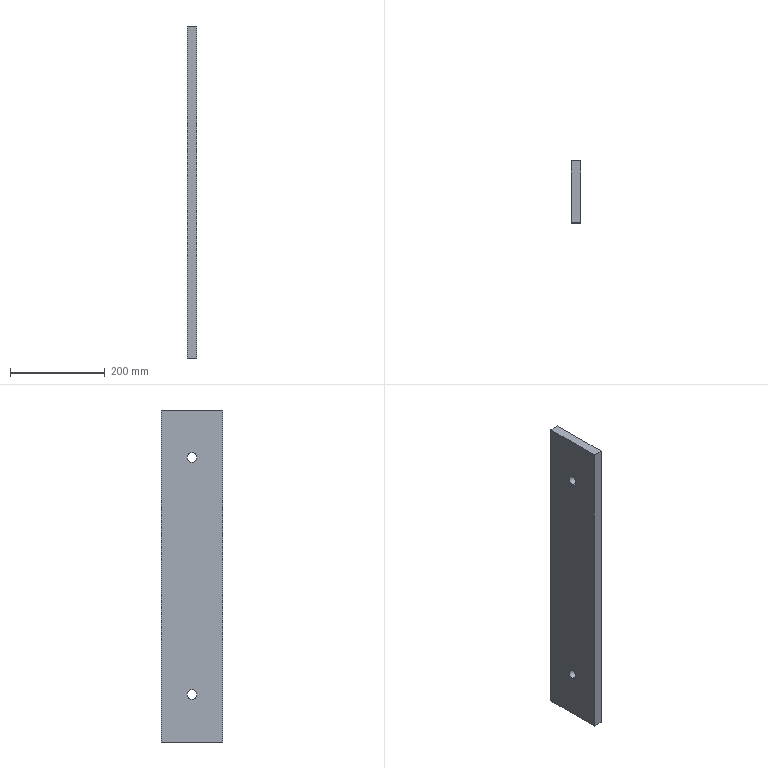Part | SolidWorks | features Extrusion 1 | 1 solid | 10 faces | box 20 x 130 x 700 mm | volume 1807434 mm3 | plane 6 | cylinder 4 | commonest cylinder face diameters 20 x4
STEP:
#1=CARTESIAN_POINT('',(20.,0.,-240.));
#2=VERTEX_POINT('',#1);
#3=CARTESIAN_POINT('',(20.,0.,-260.));
#4=VERTEX_POINT('',#3);
#5=CARTESIAN_POINT('',(20.,0.,-250.));
#6=DIRECTION('',(1.,0.,0.));
#7=DIRECTION('',(0.,0.,-1.));
#8=AXIS2_PLACEMENT_3D('',#5,#6,#7);
#9=CIRCLE('',#8,10.);
#10=EDGE_CURVE('',#2,#4,#9,.T.);
#11=ORIENTED_EDGE('',*,*,#10,.T.);
#12=CARTESIAN_POINT('',(0.,0.,-260.));
#13=VERTEX_POINT('',#12);
#14=CARTESIAN_POINT('',(20.,0.,-260.));
#15=DIRECTION('',(-1.,0.,0.));
#16=VECTOR('',#15,1000.);
#17=LINE('',#14,#16);
#18=EDGE_CURVE('',#4,#13,#17,.T.);
#19=ORIENTED_EDGE('',*,*,#18,.T.);
#20=CARTESIAN_POINT('',(0.,0.,-240.));
#21=VERTEX_POINT('',#20);
#22=CARTESIAN_POINT('',(0.,0.,-250.));
#23=DIRECTION('',(1.,0.,0.));
#24=DIRECTION('',(0.,0.,-1.));
#25=AXIS2_PLACEMENT_3D('',#22,#23,#24);
#26=CIRCLE('',#25,10.);
#27=EDGE_CURVE('',#21,#13,#26,.T.);
#28=ORIENTED_EDGE('',*,*,#27,.F.);
#29=CARTESIAN_POINT('',(20.,0.,-240.));
#30=DIRECTION('',(-1.,0.,0.));
#31=VECTOR('',#30,1000.);
#32=LINE('',#29,#31);
#33=EDGE_CURVE('',#2,#21,#32,.T.);
#34=ORIENTED_EDGE('',*,*,#33,.F.);
#35=EDGE_LOOP('',(#11,#19,#28,#34));
#36=FACE_OUTER_BOUND('',#35,.T.);
#37=CARTESIAN_POINT('',(20.,0.,-250.));
#38=DIRECTION('',(-1.,0.,0.));
#39=DIRECTION('',(0.,0.,1.));
#40=AXIS2_PLACEMENT_3D('',#37,#38,#39);
#41=CYLINDRICAL_SURFACE('',#40,10.);
#42=ADVANCED_FACE('',(#36),#41,.F.);
#43=CARTESIAN_POINT('',(20.,0.,260.));
#44=VERTEX_POINT('',#43);
#45=CARTESIAN_POINT('',(20.,0.,240.));
#46=VERTEX_POINT('',#45);
#47=CARTESIAN_POINT('',(20.,0.,250.));
#48=DIRECTION('',(1.,0.,0.));
#49=DIRECTION('',(0.,0.,-1.));
#50=AXIS2_PLACEMENT_3D('',#47,#48,#49);
#51=CIRCLE('',#50,10.);
#52=EDGE_CURVE('',#44,#46,#51,.T.);
#53=ORIENTED_EDGE('',*,*,#52,.T.);
#54=CARTESIAN_POINT('',(0.,0.,240.));
#55=VERTEX_POINT('',#54);
#56=CARTESIAN_POINT('',(20.,0.,240.));
#57=DIRECTION('',(-1.,0.,0.));
#58=VECTOR('',#57,1000.);
#59=LINE('',#56,#58);
#60=EDGE_CURVE('',#46,#55,#59,.T.);
#61=ORIENTED_EDGE('',*,*,#60,.T.);
#62=CARTESIAN_POINT('',(0.,0.,260.));
#63=VERTEX_POINT('',#62);
#64=CARTESIAN_POINT('',(0.,0.,250.));
#65=DIRECTION('',(1.,0.,0.));
#66=DIRECTION('',(0.,0.,-1.));
#67=AXIS2_PLACEMENT_3D('',#64,#65,#66);
#68=CIRCLE('',#67,10.);
#69=EDGE_CURVE('',#63,#55,#68,.T.);
#70=ORIENTED_EDGE('',*,*,#69,.F.);
#71=CARTESIAN_POINT('',(20.,0.,260.));
#72=DIRECTION('',(-1.,0.,0.));
#73=VECTOR('',#72,1000.);
#74=LINE('',#71,#73);
#75=EDGE_CURVE('',#44,#63,#74,.T.);
#76=ORIENTED_EDGE('',*,*,#75,.F.);
#77=EDGE_LOOP('',(#53,#61,#70,#76));
#78=FACE_OUTER_BOUND('',#77,.T.);
#79=CARTESIAN_POINT('',(20.,0.,250.));
#80=DIRECTION('',(-1.,0.,0.));
#81=DIRECTION('',(0.,0.,1.));
#82=AXIS2_PLACEMENT_3D('',#79,#80,#81);
#83=CYLINDRICAL_SURFACE('',#82,10.);
#84=ADVANCED_FACE('',(#78),#83,.F.);
#85=ORIENTED_EDGE('',*,*,#52,.F.);
#86=CARTESIAN_POINT('',(20.,0.,250.));
#87=DIRECTION('',(1.,0.,0.));
#88=DIRECTION('',(0.,0.,-1.));
#89=AXIS2_PLACEMENT_3D('',#86,#87,#88);
#90=CIRCLE('',#89,10.);
#91=EDGE_CURVE('',#46,#44,#90,.T.);
#92=ORIENTED_EDGE('',*,*,#91,.F.);
#93=EDGE_LOOP('',(#85,#92));
#94=FACE_BOUND('',#93,.T.);
#95=CARTESIAN_POINT('',(20.,-65.,-350.));
#96=VERTEX_POINT('',#95);
#97=CARTESIAN_POINT('',(20.,65.,-350.));
#98=VERTEX_POINT('',#97);
#99=CARTESIAN_POINT('',(20.,65.,-350.));
#100=DIRECTION('',(0.,1.,0.));
#101=VECTOR('',#100,1000.);
#102=LINE('',#99,#101);
#103=EDGE_CURVE('',#96,#98,#102,.T.);
#104=ORIENTED_EDGE('',*,*,#103,.T.);
#105=CARTESIAN_POINT('',(20.,65.,350.));
#106=VERTEX_POINT('',#105);
#107=CARTESIAN_POINT('',(20.,65.,350.));
#108=DIRECTION('',(0.,0.,1.));
#109=VECTOR('',#108,1000.);
#110=LINE('',#107,#109);
#111=EDGE_CURVE('',#98,#106,#110,.T.);
#112=ORIENTED_EDGE('',*,*,#111,.T.);
#113=CARTESIAN_POINT('',(20.,-65.,350.));
#114=VERTEX_POINT('',#113);
#115=CARTESIAN_POINT('',(20.,65.,350.));
#116=DIRECTION('',(0.,-1.,0.));
#117=VECTOR('',#116,1000.);
#118=LINE('',#115,#117);
#119=EDGE_CURVE('',#106,#114,#118,.T.);
#120=ORIENTED_EDGE('',*,*,#119,.T.);
#121=CARTESIAN_POINT('',(20.,-65.,350.));
#122=DIRECTION('',(0.,0.,-1.));
#123=VECTOR('',#122,1000.);
#124=LINE('',#121,#123);
#125=EDGE_CURVE('',#114,#96,#124,.T.);
#126=ORIENTED_EDGE('',*,*,#125,.T.);
#127=EDGE_LOOP('',(#104,#112,#120,#126));
#128=FACE_OUTER_BOUND('',#127,.T.);
#129=ORIENTED_EDGE('',*,*,#10,.F.);
#130=CARTESIAN_POINT('',(20.,0.,-250.));
#131=DIRECTION('',(1.,0.,0.));
#132=DIRECTION('',(0.,0.,-1.));
#133=AXIS2_PLACEMENT_3D('',#130,#131,#132);
#134=CIRCLE('',#133,10.);
#135=EDGE_CURVE('',#4,#2,#134,.T.);
#136=ORIENTED_EDGE('',*,*,#135,.F.);
#137=EDGE_LOOP('',(#129,#136));
#138=FACE_BOUND('',#137,.T.);
#139=CARTESIAN_POINT('',(20.,0.,0.));
#140=DIRECTION('',(1.,0.,0.));
#141=DIRECTION('',(0.,0.,-1.));
#142=AXIS2_PLACEMENT_3D('',#139,#140,#141);
#143=PLANE('',#142);
#144=ADVANCED_FACE('',(#94,#128,#138),#143,.T.);
#145=CARTESIAN_POINT('',(0.,-65.,-350.));
#146=VERTEX_POINT('',#145);
#147=CARTESIAN_POINT('',(0.,65.,-350.));
#148=VERTEX_POINT('',#147);
#149=CARTESIAN_POINT('',(0.,65.,-350.));
#150=DIRECTION('',(0.,1.,0.));
#151=VECTOR('',#150,1000.);
#152=LINE('',#149,#151);
#153=EDGE_CURVE('',#146,#148,#152,.T.);
#154=ORIENTED_EDGE('',*,*,#153,.F.);
#155=CARTESIAN_POINT('',(0.,-65.,350.));
#156=VERTEX_POINT('',#155);
#157=CARTESIAN_POINT('',(0.,-65.,350.));
#158=DIRECTION('',(0.,0.,-1.));
#159=VECTOR('',#158,1000.);
#160=LINE('',#157,#159);
#161=EDGE_CURVE('',#156,#146,#160,.T.);
#162=ORIENTED_EDGE('',*,*,#161,.F.);
#163=CARTESIAN_POINT('',(0.,65.,350.));
#164=VERTEX_POINT('',#163);
#165=CARTESIAN_POINT('',(0.,65.,350.));
#166=DIRECTION('',(0.,-1.,0.));
#167=VECTOR('',#166,1000.);
#168=LINE('',#165,#167);
#169=EDGE_CURVE('',#164,#156,#168,.T.);
#170=ORIENTED_EDGE('',*,*,#169,.F.);
#171=CARTESIAN_POINT('',(0.,65.,350.));
#172=DIRECTION('',(0.,0.,1.));
#173=VECTOR('',#172,1000.);
#174=LINE('',#171,#173);
#175=EDGE_CURVE('',#148,#164,#174,.T.);
#176=ORIENTED_EDGE('',*,*,#175,.F.);
#177=EDGE_LOOP('',(#154,#162,#170,#176));
#178=FACE_OUTER_BOUND('',#177,.T.);
#179=ORIENTED_EDGE('',*,*,#69,.T.);
#180=CARTESIAN_POINT('',(0.,0.,250.));
#181=DIRECTION('',(1.,0.,0.));
#182=DIRECTION('',(0.,0.,-1.));
#183=AXIS2_PLACEMENT_3D('',#180,#181,#182);
#184=CIRCLE('',#183,10.);
#185=EDGE_CURVE('',#55,#63,#184,.T.);
#186=ORIENTED_EDGE('',*,*,#185,.T.);
#187=EDGE_LOOP('',(#179,#186));
#188=FACE_BOUND('',#187,.T.);
#189=ORIENTED_EDGE('',*,*,#27,.T.);
#190=CARTESIAN_POINT('',(0.,0.,-250.));
#191=DIRECTION('',(1.,0.,0.));
#192=DIRECTION('',(0.,0.,-1.));
#193=AXIS2_PLACEMENT_3D('',#190,#191,#192);
#194=CIRCLE('',#193,10.);
#195=EDGE_CURVE('',#13,#21,#194,.T.);
#196=ORIENTED_EDGE('',*,*,#195,.T.);
#197=EDGE_LOOP('',(#189,#196));
#198=FACE_BOUND('',#197,.T.);
#199=CARTESIAN_POINT('',(0.,0.,0.));
#200=DIRECTION('',(1.,0.,0.));
#201=DIRECTION('',(0.,0.,-1.));
#202=AXIS2_PLACEMENT_3D('',#199,#200,#201);
#203=PLANE('',#202);
#204=ADVANCED_FACE('',(#178,#188,#198),#203,.F.);
#205=ORIENTED_EDGE('',*,*,#153,.T.);
#206=CARTESIAN_POINT('',(20.,65.,-350.));
#207=DIRECTION('',(-1.,0.,0.));
#208=VECTOR('',#207,1000.);
#209=LINE('',#206,#208);
#210=EDGE_CURVE('',#98,#148,#209,.T.);
#211=ORIENTED_EDGE('',*,*,#210,.F.);
#212=ORIENTED_EDGE('',*,*,#103,.F.);
#213=CARTESIAN_POINT('',(20.,-65.,-350.));
#214=DIRECTION('',(-1.,0.,0.));
#215=VECTOR('',#214,1000.);
#216=LINE('',#213,#215);
#217=EDGE_CURVE('',#96,#146,#216,.T.);
#218=ORIENTED_EDGE('',*,*,#217,.T.);
#219=EDGE_LOOP('',(#205,#211,#212,#218));
#220=FACE_OUTER_BOUND('',#219,.T.);
#221=CARTESIAN_POINT('',(20.,65.,-350.));
#222=DIRECTION('',(0.,0.,1.));
#223=DIRECTION('',(1.,0.,0.));
#224=AXIS2_PLACEMENT_3D('',#221,#222,#223);
#225=PLANE('',#224);
#226=ADVANCED_FACE('',(#220),#225,.F.);
#227=ORIENTED_EDGE('',*,*,#175,.T.);
#228=CARTESIAN_POINT('',(20.,65.,350.));
#229=DIRECTION('',(-1.,0.,0.));
#230=VECTOR('',#229,1000.);
#231=LINE('',#228,#230);
#232=EDGE_CURVE('',#106,#164,#231,.T.);
#233=ORIENTED_EDGE('',*,*,#232,.F.);
#234=ORIENTED_EDGE('',*,*,#111,.F.);
#235=ORIENTED_EDGE('',*,*,#210,.T.);
#236=EDGE_LOOP('',(#227,#233,#234,#235));
#237=FACE_OUTER_BOUND('',#236,.T.);
#238=CARTESIAN_POINT('',(20.,65.,350.));
#239=DIRECTION('',(0.,-1.,0.));
#240=DIRECTION('',(0.,0.,-1.));
#241=AXIS2_PLACEMENT_3D('',#238,#239,#240);
#242=PLANE('',#241);
#243=ADVANCED_FACE('',(#237),#242,.F.);
#244=ORIENTED_EDGE('',*,*,#169,.T.);
#245=CARTESIAN_POINT('',(20.,-65.,350.));
#246=DIRECTION('',(-1.,0.,0.));
#247=VECTOR('',#246,1000.);
#248=LINE('',#245,#247);
#249=EDGE_CURVE('',#114,#156,#248,.T.);
#250=ORIENTED_EDGE('',*,*,#249,.F.);
#251=ORIENTED_EDGE('',*,*,#119,.F.);
#252=ORIENTED_EDGE('',*,*,#232,.T.);
#253=EDGE_LOOP('',(#244,#250,#251,#252));
#254=FACE_OUTER_BOUND('',#253,.T.);
#255=CARTESIAN_POINT('',(20.,65.,350.));
#256=DIRECTION('',(0.,0.,-1.));
#257=DIRECTION('',(-1.,0.,0.));
#258=AXIS2_PLACEMENT_3D('',#255,#256,#257);
#259=PLANE('',#258);
#260=ADVANCED_FACE('',(#254),#259,.F.);
#261=ORIENTED_EDGE('',*,*,#161,.T.);
#262=ORIENTED_EDGE('',*,*,#217,.F.);
#263=ORIENTED_EDGE('',*,*,#125,.F.);
#264=ORIENTED_EDGE('',*,*,#249,.T.);
#265=EDGE_LOOP('',(#261,#262,#263,#264));
#266=FACE_OUTER_BOUND('',#265,.T.);
#267=CARTESIAN_POINT('',(20.,-65.,350.));
#268=DIRECTION('',(0.,1.,0.));
#269=DIRECTION('',(0.,0.,1.));
#270=AXIS2_PLACEMENT_3D('',#267,#268,#269);
#271=PLANE('',#270);
#272=ADVANCED_FACE('',(#266),#271,.F.);
#273=ORIENTED_EDGE('',*,*,#60,.F.);
#274=ORIENTED_EDGE('',*,*,#91,.T.);
#275=ORIENTED_EDGE('',*,*,#75,.T.);
#276=ORIENTED_EDGE('',*,*,#185,.F.);
#277=EDGE_LOOP('',(#273,#274,#275,#276));
#278=FACE_OUTER_BOUND('',#277,.T.);
#279=CARTESIAN_POINT('',(20.,0.,250.));
#280=DIRECTION('',(-1.,0.,0.));
#281=DIRECTION('',(0.,0.,1.));
#282=AXIS2_PLACEMENT_3D('',#279,#280,#281);
#283=CYLINDRICAL_SURFACE('',#282,10.);
#284=ADVANCED_FACE('',(#278),#283,.F.);
#285=ORIENTED_EDGE('',*,*,#18,.F.);
#286=ORIENTED_EDGE('',*,*,#135,.T.);
#287=ORIENTED_EDGE('',*,*,#33,.T.);
#288=ORIENTED_EDGE('',*,*,#195,.F.);
#289=EDGE_LOOP('',(#285,#286,#287,#288));
#290=FACE_OUTER_BOUND('',#289,.T.);
#291=CARTESIAN_POINT('',(20.,0.,-250.));
#292=DIRECTION('',(-1.,0.,0.));
#293=DIRECTION('',(0.,0.,1.));
#294=AXIS2_PLACEMENT_3D('',#291,#292,#293);
#295=CYLINDRICAL_SURFACE('',#294,10.);
#296=ADVANCED_FACE('',(#290),#295,.F.);
#297=CLOSED_SHELL('',(#42,#84,#144,#204,#226,#243,#260,#272,#284,#296));
#298=MANIFOLD_SOLID_BREP('',#297);
#299=CARTESIAN_POINT('',(0.,0.,0.));
#300=DIRECTION('',(0.,0.,1.));
#301=DIRECTION('',(1.,0.,0.));
#302=AXIS2_PLACEMENT_3D('',#299,#300,#301);
#303=(LENGTH_UNIT()NAMED_UNIT(*)SI_UNIT(.MILLI.,.METRE.));
#304=UNCERTAINTY_MEASURE_WITH_UNIT(LENGTH_MEASURE(0.00001),#303,'','');
#305=(NAMED_UNIT(*)PLANE_ANGLE_UNIT()SI_UNIT($,.RADIAN.));
#306=(NAMED_UNIT(*)SI_UNIT($,.STERADIAN.)SOLID_ANGLE_UNIT());
#307=(GEOMETRIC_REPRESENTATION_CONTEXT(3)GLOBAL_UNCERTAINTY_ASSIGNED_CONTEXT((#304))GLOBAL_UNIT_ASSIGNED_CONTEXT((#303,#305,#306))REPRESENTATION_CONTEXT('',''));
#308=ADVANCED_BREP_SHAPE_REPRESENTATION('',(#298,#302),#307);